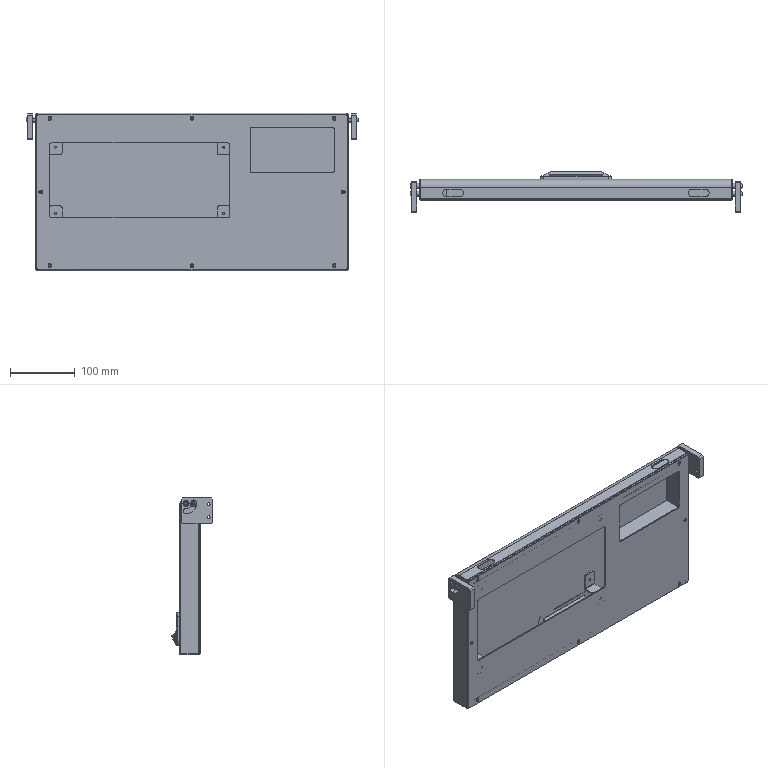Part | NX | features BREP 23 | 33 solids | 931 faces | box 513.5 x 63.5 x 244 mm | volume 365849 mm3 | plane 445 | cylinder 322 | cone 144 | spline 12 | sphere 4 | torus 4 | commonest cylinder face diameters 8 x56 6 x44 3.3 x24 4.5 x24 4.6 x22 4 x12